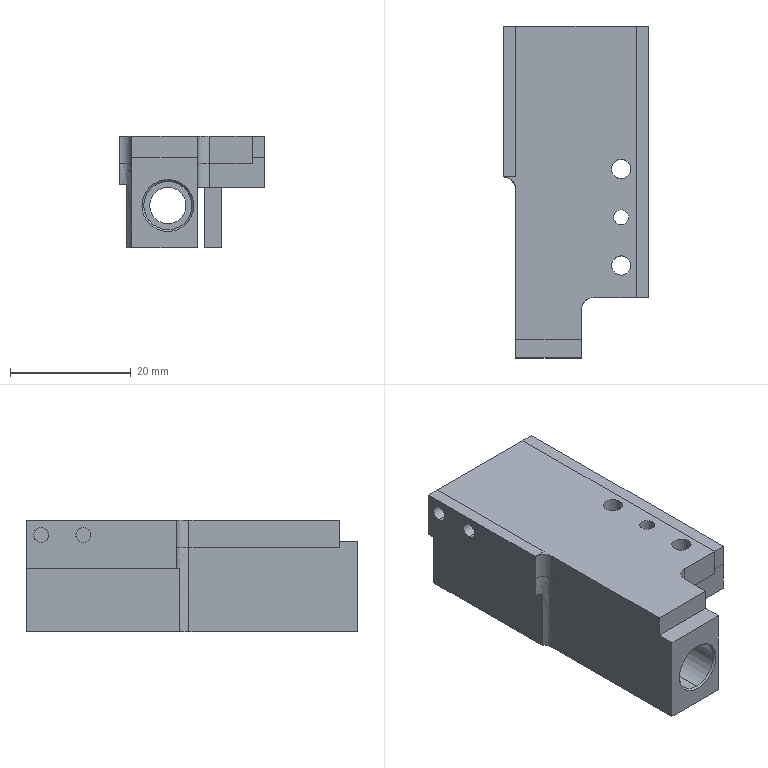NC program | NX | posted with a generic post | part box 24.15 x 55 x 18.5 mm
Whole program:
N10 G17 G21 G94 G90
(DRILLING_COPY_1 , TOOL : D6A45)
N12 T07 M6
N14 G54
N16 G17 G0 G90 X10. Y12.5 B0. C0. S5000 M3
N18 G43 Z30. H7
N20 G94 G81 G98 Z-8.775 F250. R-4.175
N22 X3.
N24 G80
N26 G0 X3. Y12.5 Z30.
N28 M5
(DRILLING_COPY_COPY_1 , TOOL : 2.5ZT)
N30 T12 M6
N32 G54
N34 G17 G0 G90 X10. Y12.5 B0. C0. S2000 M3
N36 G43 Z30. H12
N38 G94 G83 G98 Z-12.326 F120. Q2. R-4.175
N40 X3.
N42 G80
N44 G0 X3. Y12.5 Z30.
N46 M5
N48 M2